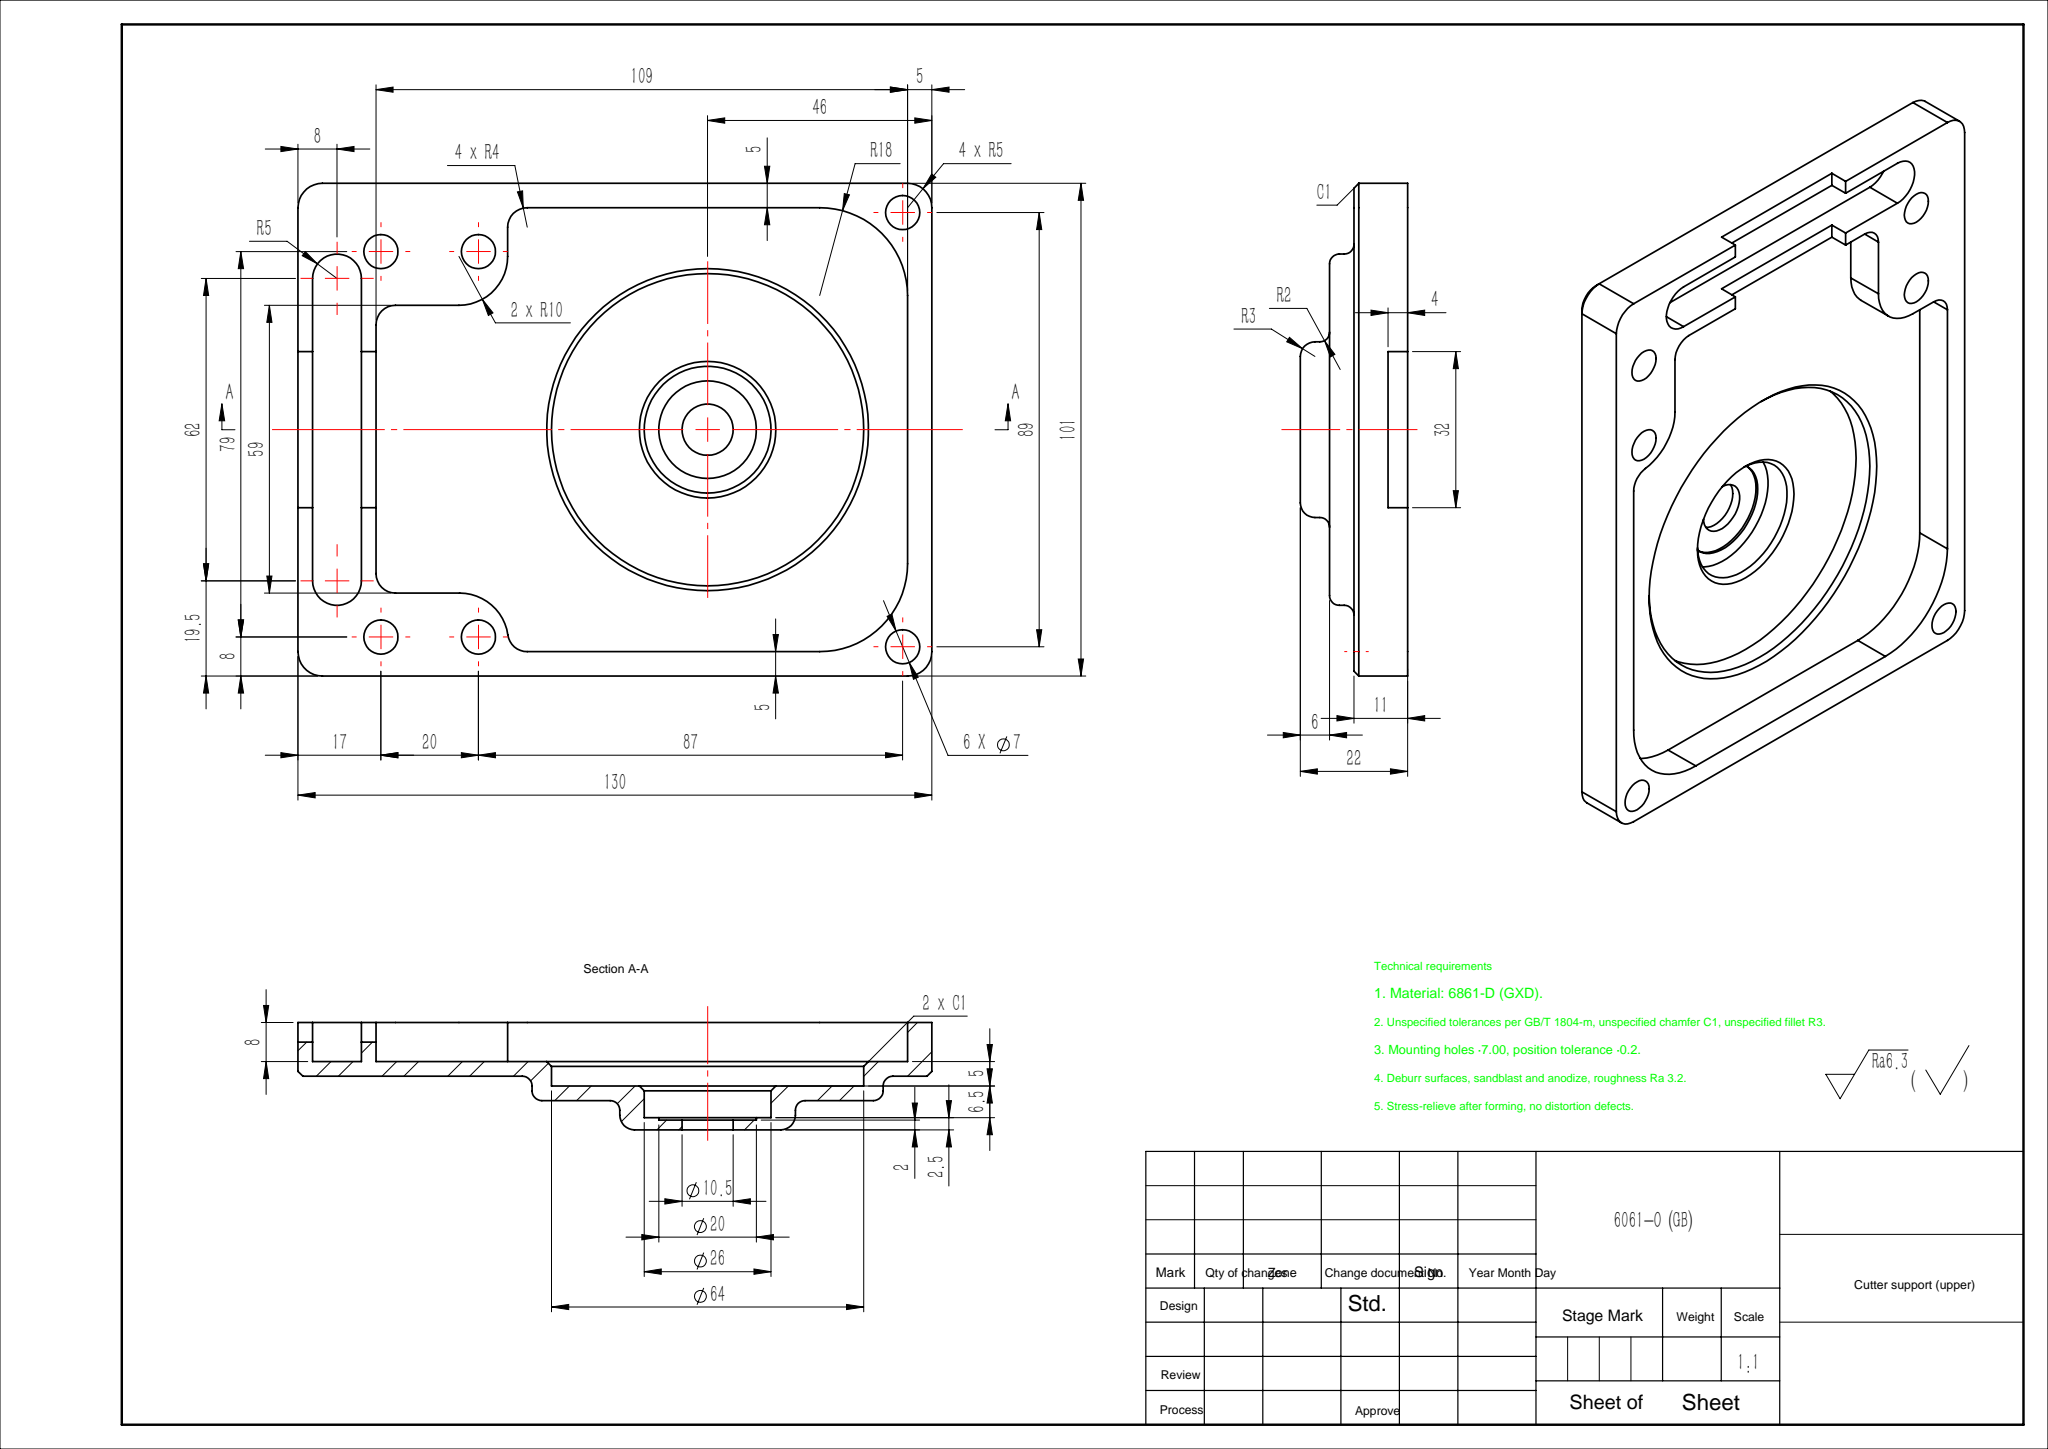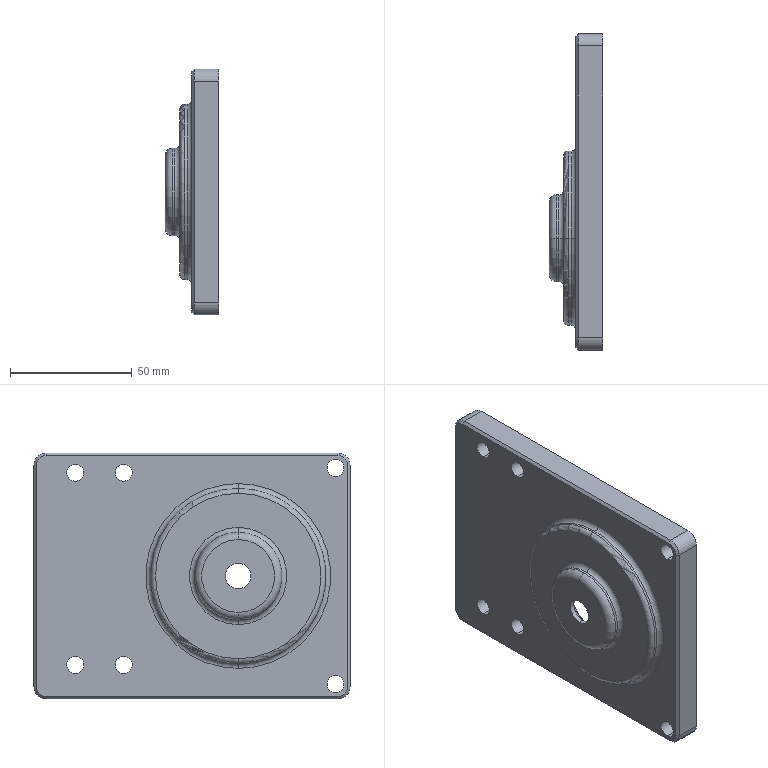Part | SolidWorks | features ICE 10, Fillet 5, Chamfer 1, Extrusion 1, HoleWzd 1 | 1 solid | 87 faces | box 22 x 130 x 101 mm | volume 69870 mm3 | cylinder 39 | plane 32 | torus 8 | cone 8 | commonest cylinder face diameters 7 x12 10 x7 8 x4 20 x4 36 x4 10.5 x2